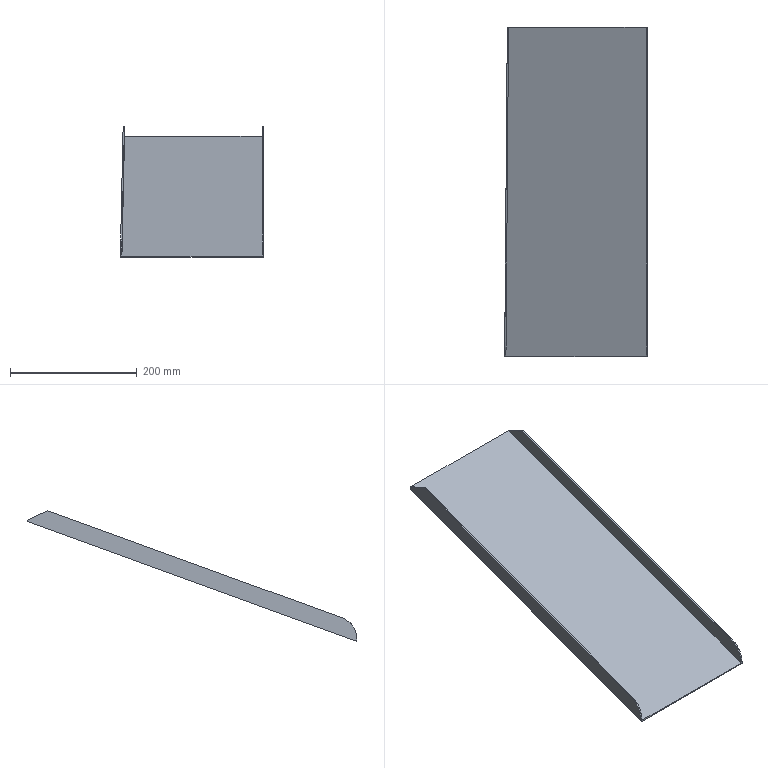Part | NX | features solid 2 | 1 solid | 14 faces | box 225.247 x 520 x 206.335 mm | volume 298449 mm3 | plane 8 | spline 5 | cylinder 1 | commonest cylinder face diameters 70 x1
STEP:
#1=CARTESIAN_POINT('',(-1188.242,-620.,-420.844));
#2=VERTEX_POINT('',#1);
#3=CARTESIAN_POINT('',(-967.,-620.,-420.844));
#4=VERTEX_POINT('',#3);
#5=CARTESIAN_POINT('',(-1490.,-620.,-420.844));
#6=DIRECTION('',(1.,0.,0.));
#7=VECTOR('',#6,1000.);
#8=LINE('',#5,#7);
#9=EDGE_CURVE('',#2,#4,#8,.T.);
#10=ORIENTED_EDGE('',*,*,#9,.T.);
#11=CARTESIAN_POINT('',(-967.,-100.,-231.58));
#12=VERTEX_POINT('',#11);
#13=CARTESIAN_POINT('',(-967.,-100.,-231.58));
#14=DIRECTION('',(0.,-0.9397,-0.342));
#15=VECTOR('',#14,1000.);
#16=LINE('',#13,#15);
#17=EDGE_CURVE('',#12,#4,#16,.T.);
#18=ORIENTED_EDGE('',*,*,#17,.F.);
#19=CARTESIAN_POINT('',(-1184.083,-100.019,-231.586));
#20=VERTEX_POINT('',#19);
#21=CARTESIAN_POINT('',(-1490.,-100.,-231.58));
#22=DIRECTION('',(1.,0.,0.));
#23=VECTOR('',#22,1000.);
#24=LINE('',#21,#23);
#25=EDGE_CURVE('',#20,#12,#24,.T.);
#26=ORIENTED_EDGE('',*,*,#25,.F.);
#27=CARTESIAN_POINT('',(-1188.242,-620.,-420.844));
#28=CARTESIAN_POINT('',(-1188.185,-612.224,-418.014));
#29=CARTESIAN_POINT('',(-1188.091,-599.128,-413.247));
#30=CARTESIAN_POINT('',(-1187.963,-581.34,-406.773));
#31=CARTESIAN_POINT('',(-1187.884,-570.46,-402.813));
#32=CARTESIAN_POINT('',(-1187.823,-561.941,-399.712));
#33=CARTESIAN_POINT('',(-1187.759,-553.064,-396.481));
#34=CARTESIAN_POINT('',(-1187.692,-543.828,-393.12));
#35=CARTESIAN_POINT('',(-1187.634,-535.833,-390.21));
#36=CARTESIAN_POINT('',(-1187.587,-529.258,-387.817));
#37=CARTESIAN_POINT('',(-1187.557,-525.074,-386.294));
#38=CARTESIAN_POINT('',(-1187.532,-521.683,-385.059));
#39=CARTESIAN_POINT('',(-1187.517,-519.544,-384.281));
#40=CARTESIAN_POINT('',(-1187.504,-517.822,-383.654));
#41=CARTESIAN_POINT('',(-1187.497,-516.74,-383.261));
#42=CARTESIAN_POINT('',(-1187.49,-515.874,-382.945));
#43=CARTESIAN_POINT('',(-1187.481,-514.573,-382.472));
#44=CARTESIAN_POINT('',(-1187.466,-512.553,-381.737));
#45=CARTESIAN_POINT('',(-1187.446,-509.692,-380.695));
#46=CARTESIAN_POINT('',(-1187.423,-506.519,-379.54));
#47=CARTESIAN_POINT('',(-1187.401,-503.548,-378.459));
#48=CARTESIAN_POINT('',(-1187.375,-499.877,-377.123));
#49=CARTESIAN_POINT('',(-1187.346,-495.82,-375.646));
#50=CARTESIAN_POINT('',(-1187.317,-491.809,-374.186));
#51=CARTESIAN_POINT('',(-1187.298,-489.18,-373.23));
#52=CARTESIAN_POINT('',(-1187.286,-487.505,-372.62));
#53=CARTESIAN_POINT('',(-1187.278,-486.462,-372.24));
#54=CARTESIAN_POINT('',(-1187.273,-485.772,-371.989));
#55=CARTESIAN_POINT('',(-1187.27,-485.382,-371.847));
#56=CARTESIAN_POINT('',(-1187.269,-485.186,-371.776));
#57=CARTESIAN_POINT('',(-1187.268,-485.054,-371.728));
#58=CARTESIAN_POINT('',(-1187.267,-484.948,-371.689));
#59=CARTESIAN_POINT('',(-1187.267,-484.886,-371.667));
#60=CARTESIAN_POINT('',(-1187.266,-484.815,-371.641));
#61=CARTESIAN_POINT('',(-1187.266,-484.839,-371.65));
#62=CARTESIAN_POINT('',(-1187.264,-484.524,-371.535));
#63=CARTESIAN_POINT('',(-1187.261,-484.132,-371.392));
#64=CARTESIAN_POINT('',(-1187.255,-483.245,-371.069));
#65=CARTESIAN_POINT('',(-1187.246,-482.064,-370.639));
#66=CARTESIAN_POINT('',(-1187.236,-480.662,-370.129));
#67=CARTESIAN_POINT('',(-1187.226,-479.309,-369.637));
#68=CARTESIAN_POINT('',(-1187.214,-477.558,-368.999));
#69=CARTESIAN_POINT('',(-1187.193,-474.64,-367.937));
#70=CARTESIAN_POINT('',(-1187.171,-471.638,-366.845));
#71=CARTESIAN_POINT('',(-1187.152,-468.97,-365.874));
#72=CARTESIAN_POINT('',(-1187.139,-467.136,-365.206));
#73=CARTESIAN_POINT('',(-1187.127,-465.468,-364.599));
#74=CARTESIAN_POINT('',(-1187.118,-464.216,-364.143));
#75=CARTESIAN_POINT('',(-1187.111,-463.299,-363.81));
#76=CARTESIAN_POINT('',(-1187.106,-462.652,-363.574));
#77=CARTESIAN_POINT('',(-1187.103,-462.15,-363.391));
#78=CARTESIAN_POINT('',(-1187.1,-461.811,-363.268));
#79=CARTESIAN_POINT('',(-1187.099,-461.632,-363.203));
#80=CARTESIAN_POINT('',(-1187.098,-461.5,-363.155));
#81=CARTESIAN_POINT('',(-1187.098,-461.448,-363.136));
#82=CARTESIAN_POINT('',(-1187.096,-461.203,-363.047));
#83=CARTESIAN_POINT('',(-1187.092,-460.733,-362.876));
#84=CARTESIAN_POINT('',(-1187.086,-459.849,-362.554));
#85=CARTESIAN_POINT('',(-1187.077,-458.631,-362.11));
#86=CARTESIAN_POINT('',(-1187.068,-457.276,-361.617));
#87=CARTESIAN_POINT('',(-1187.056,-455.599,-361.007));
#88=CARTESIAN_POINT('',(-1187.043,-453.755,-360.336));
#89=CARTESIAN_POINT('',(-1187.031,-451.936,-359.674));
#90=CARTESIAN_POINT('',(-1187.024,-450.764,-359.247));
#91=CARTESIAN_POINT('',(-1187.019,-450.,-358.969));
#92=CARTESIAN_POINT('',(-1187.017,-449.597,-358.822));
#93=CARTESIAN_POINT('',(-1187.015,-449.225,-358.687));
#94=CARTESIAN_POINT('',(-1187.012,-448.509,-358.427));
#95=CARTESIAN_POINT('',(-1187.006,-447.325,-357.995));
#96=CARTESIAN_POINT('',(-1186.998,-445.401,-357.295));
#97=CARTESIAN_POINT('',(-1186.989,-443.387,-356.562));
#98=CARTESIAN_POINT('',(-1186.982,-441.761,-355.97));
#99=CARTESIAN_POINT('',(-1186.977,-440.769,-355.609));
#100=CARTESIAN_POINT('',(-1186.974,-439.996,-355.328));
#101=CARTESIAN_POINT('',(-1186.971,-439.322,-355.083));
#102=CARTESIAN_POINT('',(-1186.969,-438.774,-354.883));
#103=CARTESIAN_POINT('',(-1186.967,-438.412,-354.751));
#104=CARTESIAN_POINT('',(-1186.966,-438.182,-354.668));
#105=CARTESIAN_POINT('',(-1186.965,-438.007,-354.604));
#106=CARTESIAN_POINT('',(-1186.965,-437.992,-354.598));
#107=CARTESIAN_POINT('',(-1186.965,-437.97,-354.59));
#108=CARTESIAN_POINT('',(-1186.965,-437.916,-354.571));
#109=CARTESIAN_POINT('',(-1186.964,-437.786,-354.524));
#110=CARTESIAN_POINT('',(-1186.963,-437.541,-354.434));
#111=CARTESIAN_POINT('',(-1186.96,-437.171,-354.3));
#112=CARTESIAN_POINT('',(-1186.957,-436.727,-354.138));
#113=CARTESIAN_POINT('',(-1186.952,-436.036,-353.886));
#114=CARTESIAN_POINT('',(-1186.945,-434.985,-353.504));
#115=CARTESIAN_POINT('',(-1186.933,-433.427,-352.937));
#116=CARTESIAN_POINT('',(-1186.918,-431.57,-352.261));
#117=CARTESIAN_POINT('',(-1186.901,-429.415,-351.477));
#118=CARTESIAN_POINT('',(-1186.881,-426.963,-350.584));
#119=CARTESIAN_POINT('',(-1186.858,-424.211,-349.583));
#120=CARTESIAN_POINT('',(-1186.837,-421.672,-348.659));
#121=CARTESIAN_POINT('',(-1186.819,-419.488,-347.864));
#122=CARTESIAN_POINT('',(-1186.807,-418.07,-347.348));
#123=CARTESIAN_POINT('',(-1186.797,-416.876,-346.913));
#124=CARTESIAN_POINT('',(-1186.792,-416.238,-346.681));
#125=CARTESIAN_POINT('',(-1186.788,-415.73,-346.496));
#126=CARTESIAN_POINT('',(-1186.786,-415.574,-346.439));
#127=CARTESIAN_POINT('',(-1186.784,-415.27,-346.328));
#128=CARTESIAN_POINT('',(-1186.779,-414.683,-346.115));
#129=CARTESIAN_POINT('',(-1186.772,-413.834,-345.806));
#130=CARTESIAN_POINT('',(-1186.761,-412.481,-345.313));
#131=CARTESIAN_POINT('',(-1186.747,-410.788,-344.697));
#132=CARTESIAN_POINT('',(-1186.713,-406.726,-343.218));
#133=CARTESIAN_POINT('',(-1186.68,-402.663,-341.74));
#134=CARTESIAN_POINT('',(-1186.647,-398.601,-340.261));
#135=CARTESIAN_POINT('',(-1186.626,-396.033,-339.327));
#136=CARTESIAN_POINT('',(-1186.589,-391.435,-337.653));
#137=CARTESIAN_POINT('',(-1186.537,-384.811,-335.242));
#138=CARTESIAN_POINT('',(-1186.484,-378.05,-332.781));
#139=CARTESIAN_POINT('',(-1186.441,-372.569,-330.787));
#140=CARTESIAN_POINT('',(-1186.415,-369.113,-329.528));
#141=CARTESIAN_POINT('',(-1186.394,-366.33,-328.516));
#142=CARTESIAN_POINT('',(-1186.378,-364.23,-327.751));
#143=CARTESIAN_POINT('',(-1186.364,-362.482,-327.115));
#144=CARTESIAN_POINT('',(-1186.355,-361.236,-326.662));
#145=CARTESIAN_POINT('',(-1186.35,-360.552,-326.413));
#146=CARTESIAN_POINT('',(-1186.345,-359.957,-326.196));
#147=CARTESIAN_POINT('',(-1186.343,-359.671,-326.092));
#148=CARTESIAN_POINT('',(-1186.339,-359.181,-325.914));
#149=CARTESIAN_POINT('',(-1186.333,-358.369,-325.618));
#150=CARTESIAN_POINT('',(-1186.324,-357.17,-325.182));
#151=CARTESIAN_POINT('',(-1186.313,-355.723,-324.655));
#152=CARTESIAN_POINT('',(-1186.298,-353.764,-323.942));
#153=CARTESIAN_POINT('',(-1186.279,-351.267,-323.033));
#154=CARTESIAN_POINT('',(-1186.247,-347.165,-321.54));
#155=CARTESIAN_POINT('',(-1186.206,-341.841,-319.603));
#156=CARTESIAN_POINT('',(-1186.153,-335.137,-317.162));
#157=CARTESIAN_POINT('',(-1186.097,-328.117,-314.607));
#158=CARTESIAN_POINT('',(-1186.018,-318.336,-311.047));
#159=CARTESIAN_POINT('',(-1185.912,-305.321,-306.31));
#160=CARTESIAN_POINT('',(-1185.773,-288.44,-300.166));
#161=CARTESIAN_POINT('',(-1185.647,-273.321,-294.663));
#162=CARTESIAN_POINT('',(-1185.54,-260.594,-290.031));
#163=CARTESIAN_POINT('',(-1185.47,-252.378,-287.041));
#164=CARTESIAN_POINT('',(-1185.413,-245.645,-284.59));
#165=CARTESIAN_POINT('',(-1185.369,-240.522,-282.725));
#166=CARTESIAN_POINT('',(-1185.332,-236.169,-281.141));
#167=CARTESIAN_POINT('',(-1185.302,-232.688,-279.874));
#168=CARTESIAN_POINT('',(-1185.279,-229.946,-278.876));
#169=CARTESIAN_POINT('',(-1185.259,-227.609,-278.025));
#170=CARTESIAN_POINT('',(-1185.232,-224.394,-276.855));
#171=CARTESIAN_POINT('',(-1185.185,-218.917,-274.862));
#172=CARTESIAN_POINT('',(-1185.12,-211.308,-272.092));
#173=CARTESIAN_POINT('',(-1185.045,-202.59,-268.919));
#174=CARTESIAN_POINT('',(-1184.973,-194.265,-265.889));
#175=CARTESIAN_POINT('',(-1184.905,-186.34,-263.005));
#176=CARTESIAN_POINT('',(-1184.851,-180.067,-260.721));
#177=CARTESIAN_POINT('',(-1184.809,-175.246,-258.967));
#178=CARTESIAN_POINT('',(-1184.779,-171.733,-257.688));
#179=CARTESIAN_POINT('',(-1184.754,-168.88,-256.65));
#180=CARTESIAN_POINT('',(-1184.737,-166.942,-255.944));
#181=CARTESIAN_POINT('',(-1184.728,-165.824,-255.537));
#182=CARTESIAN_POINT('',(-1184.721,-165.057,-255.258));
#183=CARTESIAN_POINT('',(-1184.712,-164.044,-254.89));
#184=CARTESIAN_POINT('',(-1184.701,-162.776,-254.428));
#185=CARTESIAN_POINT('',(-1184.681,-160.512,-253.604));
#186=CARTESIAN_POINT('',(-1184.641,-155.987,-251.957));
#187=CARTESIAN_POINT('',(-1184.581,-149.441,-249.575));
#188=CARTESIAN_POINT('',(-1184.506,-141.482,-246.678));
#189=CARTESIAN_POINT('',(-1184.402,-130.722,-242.761));
#190=CARTESIAN_POINT('',(-1184.264,-116.998,-237.766));
#191=CARTESIAN_POINT('',(-1184.145,-105.728,-233.664));
#192=CARTESIAN_POINT('',(-1184.083,-100.019,-231.586));
#193=B_SPLINE_CURVE_WITH_KNOTS('',3,(#27,#28,#29,#30,#31,#32,#33,#34,#35,#36,#37,#38,#39,#40,#41,#42,#43,#44,#45,#46,#47,#48,#49,#50,#51,#52,#53,#54,#55,#56,#57,#58,#59,#60,#61,#62,#63,#64,#65,#66,#67,#68,#69,#70,#71,#72,#73,#74,#75,#76,#77,#78,#79,#80,#81,#82,#83,#84,#85,#86,#87,#88,#89,#90,#91,#92,#93,#94,#95,#96,#97,#98,#99,#100,#101,#102,#103,#104,#105,#106,#107,#108,#109,#110,#111,#112,#113,#114,#115,#116,#117,#118,#119,#120,#121,#122,#123,#124,#125,#126,#127,#128,#129,#130,#131,#132,#133,#134,#135,#136,#137,#138,#139,#140,#141,#142,#143,#144,#145,#146,#147,#148,#149,#150,#151,#152,#153,#154,#155,#156,#157,#158,#159,#160,#161,#162,#163,#164,#165,#166,#167,#168,#169,#170,#171,#172,#173,#174,#175,#176,#177,#178,#179,#180,#181,#182,#183,#184,#185,#186,#187,#188,#189,#190,#191,#192),.UNSPECIFIED.,.F.,.F.,(4,1,1,1,1,1,1,1,1,1,1,1,1,1,1,1,1,1,1,1,1,1,1,1,1,1,1,1,1,1,1,1,1,1,1,1,1,1,1,1,1,1,1,1,1,1,1,1,1,1,1,1,1,1,1,1,1,1,1,1,1,1,1,1,1,1,1,1,1,1,1,1,1,1,1,1,1,1,1,1,1,1,1,1,1,1,1,1,1,1,1,1,1,1,1,1,1,1,1,1,1,1,1,1,1,1,1,1,1,1,1,1,1,1,1,1,1,1,1,1,1,1,1,1,1,1,1,1,1,1,1,1,1,1,1,1,1,1,1,1,1,1,1,1,1,1,1,1,1,1,1,1,1,1,1,1,1,1,1,1,1,1,1,4),(0.,0.0625,0.09375,0.1094,0.125,0.1406,0.1562,0.1719,0.1797,0.1875,0.1914,0.1953,0.1973,0.1992,0.2002,0.2012,0.2031,0.207,0.2109,0.2148,0.2188,0.2266,0.2344,0.2422,0.2461,0.25,0.2539,0.2559,0.2568,0.2578,0.2588,0.2593,0.2598,0.26,0.2603,0.2607,0.2617,0.2637,0.2656,0.2676,0.2695,0.2734,0.2812,0.2852,0.2891,0.293,0.2969,0.2988,0.3008,0.3027,0.3037,0.3042,0.3047,0.3049,0.3052,0.3057,0.3066,0.3086,0.3105,0.3125,0.3164,0.3203,0.3242,0.3262,0.3281,0.3301,0.332,0.3359,0.3398,0.3438,0.3457,0.3467,0.3477,0.3486,0.3491,0.3496,0.3499,0.35,0.3501,0.3503,0.3506,0.3516,0.3535,0.3555,0.3574,0.3594,0.3633,0.3672,0.3711,0.375,0.3789,0.3828,0.3867,0.3887,0.3906,0.3916,0.3926,0.3928,0.3931,0.3936,0.3945,0.3965,0.3984,0.4023,0.4062,0.4219,0.4258,0.4297,0.4375,0.4531,0.4688,0.4766,0.4844,0.4883,0.4922,0.4961,0.498,0.499,0.5,0.501,0.502,0.5039,0.5078,0.5117,0.5156,0.5234,0.5312,0.5469,0.5625,0.5781,0.5938,0.625,0.6562,0.6875,0.7031,0.7188,0.7266,0.7344,0.7422,0.7461,0.75,0.7539,0.7578,0.7656,0.7812,0.7969,0.8125,0.8281,0.8438,0.8516,0.8594,0.8672,0.8711,0.873,0.875,0.877,0.8789,0.8828,0.8906,0.9062,0.9219,0.9375,0.9688,1.),.UNSPECIFIED.);
#194=EDGE_CURVE('',#20,#2,#193,.F.);
#195=ORIENTED_EDGE('',*,*,#194,.T.);
#196=EDGE_LOOP('',(#10,#18,#26,#195));
#197=FACE_BOUND('',#196,.T.);
#198=CARTESIAN_POINT('',(-1490.,-63.022,-218.121));
#199=DIRECTION('',(0.,0.342,-0.9397));
#200=DIRECTION('',(-1.,0.,0.));
#201=AXIS2_PLACEMENT_3D('',#198,#199,#200);
#202=PLANE('',#201);
#203=ADVANCED_FACE('',(#197),#202,.F.);
#204=CARTESIAN_POINT('',(-965.,-620.,-418.747));
#205=VERTEX_POINT('',#204);
#206=CARTESIAN_POINT('',(-965.,-620.,-422.972));
#207=VERTEX_POINT('',#206);
#208=CARTESIAN_POINT('',(-965.,-620.,-570.));
#209=DIRECTION('',(0.,0.,-1.));
#210=VECTOR('',#209,1000.);
#211=LINE('',#208,#210);
#212=EDGE_CURVE('',#205,#207,#211,.T.);
#213=ORIENTED_EDGE('',*,*,#212,.F.);
#214=CARTESIAN_POINT('',(-967.,-620.,-418.747));
#215=VERTEX_POINT('',#214);
#216=CARTESIAN_POINT('',(50.,-620.,-418.747));
#217=DIRECTION('',(-1.,0.,0.));
#218=VECTOR('',#217,1000.);
#219=LINE('',#216,#218);
#220=EDGE_CURVE('',#205,#215,#219,.T.);
#221=ORIENTED_EDGE('',*,*,#220,.T.);
#222=CARTESIAN_POINT('',(-967.,-620.,-570.));
#223=DIRECTION('',(0.,0.,1.));
#224=VECTOR('',#223,1000.);
#225=LINE('',#222,#224);
#226=EDGE_CURVE('',#4,#215,#225,.T.);
#227=ORIENTED_EDGE('',*,*,#226,.F.);
#228=ORIENTED_EDGE('',*,*,#9,.F.);
#229=CARTESIAN_POINT('',(-1188.237,-620.,-418.747));
#230=VERTEX_POINT('',#229);
#231=CARTESIAN_POINT('',(-1188.242,-620.,-420.844));
#232=CARTESIAN_POINT('',(-1188.24,-620.,-420.145));
#233=CARTESIAN_POINT('',(-1188.238,-620.,-419.446));
#234=CARTESIAN_POINT('',(-1188.237,-620.,-418.747));
#235=B_SPLINE_CURVE_WITH_KNOTS('',3,(#231,#232,#233,#234),.UNSPECIFIED.,.F.,.F.,(4,4),(0.,0.002097),.UNSPECIFIED.);
#236=EDGE_CURVE('',#2,#230,#235,.T.);
#237=ORIENTED_EDGE('',*,*,#236,.T.);
#238=CARTESIAN_POINT('',(-1190.237,-620.,-418.747));
#239=VERTEX_POINT('',#238);
#240=CARTESIAN_POINT('',(-1188.237,-620.,-418.747));
#241=CARTESIAN_POINT('',(-1188.903,-620.,-418.747));
#242=CARTESIAN_POINT('',(-1189.57,-620.,-418.747));
#243=CARTESIAN_POINT('',(-1190.237,-620.,-418.747));
#244=B_SPLINE_CURVE_WITH_KNOTS('',3,(#240,#241,#242,#243),.UNSPECIFIED.,.F.,.F.,(4,4),(0.,0.002),.UNSPECIFIED.);
#245=EDGE_CURVE('',#230,#239,#244,.T.);
#246=ORIENTED_EDGE('',*,*,#245,.T.);
#247=CARTESIAN_POINT('',(-1190.247,-620.,-422.972));
#248=VERTEX_POINT('',#247);
#249=CARTESIAN_POINT('',(-1190.237,-620.,-418.747));
#250=CARTESIAN_POINT('',(-1190.24,-620.,-420.155));
#251=CARTESIAN_POINT('',(-1190.243,-620.,-421.564));
#252=CARTESIAN_POINT('',(-1190.247,-620.,-422.972));
#253=B_SPLINE_CURVE_WITH_KNOTS('',3,(#249,#250,#251,#252),.UNSPECIFIED.,.F.,.F.,(4,4),(-0.002097,0.002128),.UNSPECIFIED.);
#254=EDGE_CURVE('',#239,#248,#253,.T.);
#255=ORIENTED_EDGE('',*,*,#254,.T.);
#256=CARTESIAN_POINT('',(-1490.,-620.,-422.972));
#257=DIRECTION('',(1.,0.,0.));
#258=VECTOR('',#257,1000.);
#259=LINE('',#256,#258);
#260=EDGE_CURVE('',#248,#207,#259,.T.);
#261=ORIENTED_EDGE('',*,*,#260,.T.);
#262=EDGE_LOOP('',(#213,#221,#227,#228,#237,#246,#255,#261));
#263=FACE_BOUND('',#262,.T.);
#264=CARTESIAN_POINT('',(50.,-620.,-570.));
#265=DIRECTION('',(0.,1.,0.));
#266=DIRECTION('',(-1.,0.,0.));
#267=AXIS2_PLACEMENT_3D('',#264,#265,#266);
#268=PLANE('',#267);
#269=ADVANCED_FACE('',(#263),#268,.F.);
#270=CARTESIAN_POINT('',(-965.,-100.,-231.58));
#271=VERTEX_POINT('',#270);
#272=CARTESIAN_POINT('',(-965.,-100.,-233.708));
#273=VERTEX_POINT('',#272);
#274=CARTESIAN_POINT('',(-965.,-100.,0.));
#275=DIRECTION('',(0.,0.,-1.));
#276=VECTOR('',#275,1000.);
#277=LINE('',#274,#276);
#278=EDGE_CURVE('',#271,#273,#277,.T.);
#279=ORIENTED_EDGE('',*,*,#278,.F.);
#280=CARTESIAN_POINT('',(-965.,-132.043,-216.638));
#281=VERTEX_POINT('',#280);
#282=CARTESIAN_POINT('',(-965.,360.26,-446.202));
#283=DIRECTION('',(0.,0.9063,-0.4226));
#284=VECTOR('',#283,1000.);
#285=LINE('',#282,#284);
#286=EDGE_CURVE('',#271,#281,#285,.F.);
#287=ORIENTED_EDGE('',*,*,#286,.T.);
#288=CARTESIAN_POINT('',(-965.,-596.971,-385.858));
#289=VERTEX_POINT('',#288);
#290=CARTESIAN_POINT('',(-965.,-108.551,-208.087));
#291=DIRECTION('',(0.,-0.9397,-0.342));
#292=VECTOR('',#291,1000.);
#293=LINE('',#290,#292);
#294=EDGE_CURVE('',#281,#289,#293,.T.);
#295=ORIENTED_EDGE('',*,*,#294,.T.);
#296=CARTESIAN_POINT('',(-965.,-585.,-418.747));
#297=DIRECTION('',(1.,0.,0.));
#298=DIRECTION('',(0.,0.,-1.));
#299=AXIS2_PLACEMENT_3D('',#296,#297,#298);
#300=CIRCLE('',#299,35.);
#301=EDGE_CURVE('',#289,#205,#300,.T.);
#302=ORIENTED_EDGE('',*,*,#301,.T.);
#303=ORIENTED_EDGE('',*,*,#212,.T.);
#304=CARTESIAN_POINT('',(-965.,575.567,12.179));
#305=DIRECTION('',(0.,0.9397,0.342));
#306=VECTOR('',#305,1000.);
#307=LINE('',#304,#306);
#308=EDGE_CURVE('',#273,#207,#307,.F.);
#309=ORIENTED_EDGE('',*,*,#308,.F.);
#310=EDGE_LOOP('',(#279,#287,#295,#302,#303,#309));
#311=FACE_BOUND('',#310,.T.);
#312=CARTESIAN_POINT('',(-965.,574.883,14.058));
#313=DIRECTION('',(1.,0.,0.));
#314=DIRECTION('',(0.,0.,-1.));
#315=AXIS2_PLACEMENT_3D('',#312,#313,#314);
#316=PLANE('',#315);
#317=ADVANCED_FACE('',(#311),#316,.T.);
#318=CARTESIAN_POINT('',(-1186.09,-100.,-233.708));
#319=VERTEX_POINT('',#318);
#320=CARTESIAN_POINT('',(-1490.,-100.,-233.708));
#321=DIRECTION('',(1.,0.,0.));
#322=VECTOR('',#321,1000.);
#323=LINE('',#320,#322);
#324=EDGE_CURVE('',#319,#273,#323,.T.);
#325=ORIENTED_EDGE('',*,*,#324,.F.);
#326=CARTESIAN_POINT('',(-1186.083,-100.,-231.58));
#327=VERTEX_POINT('',#326);
#328=CARTESIAN_POINT('',(-1186.083,-100.,-231.58));
#329=CARTESIAN_POINT('',(-1186.085,-100.,-232.289));
#330=CARTESIAN_POINT('',(-1186.088,-100.,-232.998));
#331=CARTESIAN_POINT('',(-1186.09,-100.,-233.708));
#332=B_SPLINE_CURVE_WITH_KNOTS('',3,(#328,#329,#330,#331),.UNSPECIFIED.,.F.,.F.,(4,4),(0.,0.002128),.UNSPECIFIED.);
#333=EDGE_CURVE('',#327,#319,#332,.T.);
#334=ORIENTED_EDGE('',*,*,#333,.F.);
#335=CARTESIAN_POINT('',(-1186.083,-100.,-231.58));
#336=CARTESIAN_POINT('',(-1185.416,-100.,-231.58));
#337=CARTESIAN_POINT('',(-1184.749,-100.,-231.58));
#338=CARTESIAN_POINT('',(-1184.083,-100.,-231.58));
#339=B_SPLINE_CURVE_WITH_KNOTS('',3,(#335,#336,#337,#338),.UNSPECIFIED.,.F.,.F.,(4,4),(0.,1.),.UNSPECIFIED.);
#340=EDGE_CURVE('',#327,#20,#339,.T.);
#341=ORIENTED_EDGE('',*,*,#340,.T.);
#342=ORIENTED_EDGE('',*,*,#25,.T.);
#343=CARTESIAN_POINT('',(-965.,-100.,-231.58));
#344=DIRECTION('',(1.,0.,0.));
#345=VECTOR('',#344,1000.);
#346=LINE('',#343,#345);
#347=EDGE_CURVE('',#271,#12,#346,.F.);
#348=ORIENTED_EDGE('',*,*,#347,.F.);
#349=ORIENTED_EDGE('',*,*,#278,.T.);
#350=EDGE_LOOP('',(#325,#334,#341,#342,#348,#349));
#351=FACE_BOUND('',#350,.T.);
#352=CARTESIAN_POINT('',(2540.,-100.,0.));
#353=DIRECTION('',(0.,1.,0.));
#354=DIRECTION('',(0.,0.,1.));
#355=AXIS2_PLACEMENT_3D('',#352,#353,#354);
#356=PLANE('',#355);
#357=ADVANCED_FACE('',(#351),#356,.T.);
#358=CARTESIAN_POINT('',(-1186.09,-100.,-233.708));
#359=CARTESIAN_POINT('',(-1186.151,-105.657,-235.767));
#360=CARTESIAN_POINT('',(-1186.27,-116.851,-239.841));
#361=CARTESIAN_POINT('',(-1186.435,-133.279,-245.82));
#362=CARTESIAN_POINT('',(-1186.563,-146.678,-250.697));
#363=CARTESIAN_POINT('',(-1186.646,-155.88,-254.047));
#364=CARTESIAN_POINT('',(-1186.693,-161.123,-255.955));
#365=CARTESIAN_POINT('',(-1186.726,-164.949,-257.347));
#366=CARTESIAN_POINT('',(-1186.762,-169.075,-258.849));
#367=CARTESIAN_POINT('',(-1186.808,-174.471,-260.813));
#368=CARTESIAN_POINT('',(-1186.89,-183.963,-264.268));
#369=CARTESIAN_POINT('',(-1186.983,-194.79,-268.209));
#370=CARTESIAN_POINT('',(-1187.077,-205.624,-272.152));
#371=CARTESIAN_POINT('',(-1187.135,-212.395,-274.616));
#372=CARTESIAN_POINT('',(-1187.181,-217.811,-276.588));
#373=CARTESIAN_POINT('',(-1187.21,-221.197,-277.82));
#374=CARTESIAN_POINT('',(-1187.233,-223.906,-278.806));
#375=CARTESIAN_POINT('',(-1187.251,-225.935,-279.544));
#376=CARTESIAN_POINT('',(-1187.265,-227.634,-280.163));
#377=CARTESIAN_POINT('',(-1187.275,-228.807,-280.59));
#378=CARTESIAN_POINT('',(-1187.281,-229.503,-280.843));
#379=CARTESIAN_POINT('',(-1187.285,-229.953,-281.007));
#380=CARTESIAN_POINT('',(-1187.291,-230.676,-281.27));
#381=CARTESIAN_POINT('',(-1187.299,-231.543,-281.586));
#382=CARTESIAN_POINT('',(-1187.312,-233.1,-282.152));
#383=CARTESIAN_POINT('',(-1187.331,-235.289,-282.949));
#384=CARTESIAN_POINT('',(-1187.353,-237.906,-283.902));
#385=CARTESIAN_POINT('',(-1187.382,-241.366,-285.161));
#386=CARTESIAN_POINT('',(-1187.419,-245.642,-286.717));
#387=CARTESIAN_POINT('',(-1187.476,-252.377,-289.169));
#388=CARTESIAN_POINT('',(-1187.545,-260.598,-292.161));
#389=CARTESIAN_POINT('',(-1187.626,-270.148,-295.637));
#390=CARTESIAN_POINT('',(-1187.703,-279.38,-298.997));
#391=CARTESIAN_POINT('',(-1187.802,-291.269,-303.324));
#392=CARTESIAN_POINT('',(-1187.918,-305.338,-308.445));
#393=CARTESIAN_POINT('',(-1188.024,-318.352,-313.182));
#394=CARTESIAN_POINT('',(-1188.103,-328.13,-316.741));
#395=CARTESIAN_POINT('',(-1188.159,-335.148,-319.295));
#396=CARTESIAN_POINT('',(-1188.211,-341.848,-321.733));
#397=CARTESIAN_POINT('',(-1188.253,-347.168,-323.67));
#398=CARTESIAN_POINT('',(-1188.284,-351.266,-325.161));
#399=CARTESIAN_POINT('',(-1188.303,-353.761,-326.069));
#400=CARTESIAN_POINT('',(-1188.318,-355.719,-326.782));
#401=CARTESIAN_POINT('',(-1188.329,-357.164,-327.308));
#402=CARTESIAN_POINT('',(-1188.338,-358.361,-327.743));
#403=CARTESIAN_POINT('',(-1188.345,-359.173,-328.039));
#404=CARTESIAN_POINT('',(-1188.348,-359.661,-328.217));
#405=CARTESIAN_POINT('',(-1188.35,-359.953,-328.323));
#406=CARTESIAN_POINT('',(-1188.355,-360.518,-328.529));
#407=CARTESIAN_POINT('',(-1188.36,-361.177,-328.768));
#408=CARTESIAN_POINT('',(-1188.369,-362.373,-329.204));
#409=CARTESIAN_POINT('',(-1188.381,-364.06,-329.818));
#410=CARTESIAN_POINT('',(-1188.397,-366.093,-330.558));
#411=CARTESIAN_POINT('',(-1188.418,-368.801,-331.543));
#412=CARTESIAN_POINT('',(-1188.444,-372.186,-332.776));
#413=CARTESIAN_POINT('',(-1188.485,-377.603,-334.747));
#414=CARTESIAN_POINT('',(-1188.538,-384.374,-337.211));
#415=CARTESIAN_POINT('',(-1188.603,-392.499,-340.169));
#416=CARTESIAN_POINT('',(-1188.669,-400.624,-343.126));
#417=CARTESIAN_POINT('',(-1188.735,-408.749,-346.083));
#418=CARTESIAN_POINT('',(-1188.792,-415.52,-348.548));
#419=CARTESIAN_POINT('',(-1188.837,-420.936,-350.519));
#420=CARTESIAN_POINT('',(-1188.866,-424.322,-351.751));
#421=CARTESIAN_POINT('',(-1188.889,-427.03,-352.737));
#422=CARTESIAN_POINT('',(-1188.906,-429.061,-353.476));
#423=CARTESIAN_POINT('',(-1188.921,-430.754,-354.093));
#424=CARTESIAN_POINT('',(-1188.933,-432.107,-354.585));
#425=CARTESIAN_POINT('',(-1188.94,-432.957,-354.894));
#426=CARTESIAN_POINT('',(-1188.945,-433.544,-355.108));
#427=CARTESIAN_POINT('',(-1188.948,-433.891,-355.234));
#428=CARTESIAN_POINT('',(-1188.95,-434.081,-355.303));
#429=CARTESIAN_POINT('',(-1188.951,-434.294,-355.381));
#430=CARTESIAN_POINT('',(-1188.951,-434.288,-355.379));
#431=CARTESIAN_POINT('',(-1188.952,-434.328,-355.393));
#432=CARTESIAN_POINT('',(-1188.952,-434.427,-355.429));
#433=CARTESIAN_POINT('',(-1188.954,-434.715,-355.534));
#434=CARTESIAN_POINT('',(-1188.957,-435.446,-355.8));
#435=CARTESIAN_POINT('',(-1188.962,-436.601,-356.221));
#436=CARTESIAN_POINT('',(-1188.969,-438.175,-356.794));
#437=CARTESIAN_POINT('',(-1188.975,-439.568,-357.301));
#438=CARTESIAN_POINT('',(-1188.981,-440.896,-357.784));
#439=CARTESIAN_POINT('',(-1188.986,-442.082,-358.215));
#440=CARTESIAN_POINT('',(-1188.989,-442.825,-358.486));
#441=CARTESIAN_POINT('',(-1188.992,-443.541,-358.747));
#442=CARTESIAN_POINT('',(-1188.993,-443.929,-358.888));
#443=CARTESIAN_POINT('',(-1188.997,-444.65,-359.15));
#444=CARTESIAN_POINT('',(-1189.003,-446.013,-359.646));
#445=CARTESIAN_POINT('',(-1189.012,-447.859,-360.318));
#446=CARTESIAN_POINT('',(-1189.022,-449.875,-361.052));
#447=CARTESIAN_POINT('',(-1189.03,-451.244,-361.55));
#448=CARTESIAN_POINT('',(-1189.036,-452.099,-361.861));
#449=CARTESIAN_POINT('',(-1189.038,-452.44,-361.986));
#450=CARTESIAN_POINT('',(-1189.04,-452.719,-362.087));
#451=CARTESIAN_POINT('',(-1189.041,-452.893,-362.151));
#452=CARTESIAN_POINT('',(-1189.041,-452.867,-362.141));
#453=CARTESIAN_POINT('',(-1189.041,-452.934,-362.165));
#454=CARTESIAN_POINT('',(-1189.042,-453.039,-362.203));
#455=CARTESIAN_POINT('',(-1189.044,-453.311,-362.302));
#456=CARTESIAN_POINT('',(-1189.047,-453.681,-362.437));
#457=CARTESIAN_POINT('',(-1189.054,-454.639,-362.786));
#458=CARTESIAN_POINT('',(-1189.07,-456.868,-363.597));
#459=CARTESIAN_POINT('',(-1189.098,-460.757,-365.013));
#460=CARTESIAN_POINT('',(-1189.126,-464.72,-366.455));
#461=CARTESIAN_POINT('',(-1189.147,-467.539,-367.481));
#462=CARTESIAN_POINT('',(-1189.162,-469.719,-368.275));
#463=CARTESIAN_POINT('',(-1189.17,-470.827,-368.678));
#464=CARTESIAN_POINT('',(-1189.175,-471.519,-368.93));
#465=CARTESIAN_POINT('',(-1189.177,-471.771,-369.021));
#466=CARTESIAN_POINT('',(-1189.18,-472.236,-369.191));
#467=CARTESIAN_POINT('',(-1189.185,-472.897,-369.431));
#468=CARTESIAN_POINT('',(-1189.191,-473.751,-369.742));
#469=CARTESIAN_POINT('',(-1189.199,-474.764,-370.111));
#470=CARTESIAN_POINT('',(-1189.208,-476.12,-370.604));
#471=CARTESIAN_POINT('',(-1189.221,-477.812,-371.22));
#472=CARTESIAN_POINT('',(-1189.235,-479.843,-371.96));
#473=CARTESIAN_POINT('',(-1189.255,-482.552,-372.945));
#474=CARTESIAN_POINT('',(-1189.279,-485.937,-374.178));
#475=CARTESIAN_POINT('',(-1189.318,-491.354,-376.149));
#476=CARTESIAN_POINT('',(-1189.367,-498.125,-378.613));
#477=CARTESIAN_POINT('',(-1189.445,-508.958,-382.556));
#478=CARTESIAN_POINT('',(-1189.543,-522.5,-387.485));
#479=CARTESIAN_POINT('',(-1189.66,-538.75,-393.4));
#480=CARTESIAN_POINT('',(-1189.817,-560.417,-401.286));
#481=CARTESIAN_POINT('',(-1190.012,-587.5,-411.143));
#482=CARTESIAN_POINT('',(-1190.168,-609.167,-419.029));
#483=CARTESIAN_POINT('',(-1190.247,-620.,-422.972));
#484=B_SPLINE_CURVE_WITH_KNOTS('',3,(#358,#359,#360,#361,#362,#363,#364,#365,#366,#367,#368,#369,#370,#371,#372,#373,#374,#375,#376,#377,#378,#379,#380,#381,#382,#383,#384,#385,#386,#387,#388,#389,#390,#391,#392,#393,#394,#395,#396,#397,#398,#399,#400,#401,#402,#403,#404,#405,#406,#407,#408,#409,#410,#411,#412,#413,#414,#415,#416,#417,#418,#419,#420,#421,#422,#423,#424,#425,#426,#427,#428,#429,#430,#431,#432,#433,#434,#435,#436,#437,#438,#439,#440,#441,#442,#443,#444,#445,#446,#447,#448,#449,#450,#451,#452,#453,#454,#455,#456,#457,#458,#459,#460,#461,#462,#463,#464,#465,#466,#467,#468,#469,#470,#471,#472,#473,#474,#475,#476,#477,#478,#479,#480,#481,#482,#483),.UNSPECIFIED.,.F.,.F.,(4,1,1,1,1,1,1,1,1,1,1,1,1,1,1,1,1,1,1,1,1,1,1,1,1,1,1,1,1,1,1,1,1,1,1,1,1,1,1,1,1,1,1,1,1,1,1,1,1,1,1,1,1,1,1,1,1,1,1,1,1,1,1,1,1,1,1,1,1,1,1,1,1,1,1,1,1,1,1,1,1,1,1,1,1,1,1,1,1,1,1,1,1,1,1,1,1,1,1,1,1,1,1,1,1,1,1,1,1,1,1,1,1,1,1,1,1,1,1,1,1,1,1,4),(0.,0.03125,0.0625,0.09375,0.1094,0.1172,0.125,0.1328,0.1406,0.1562,0.1875,0.2031,0.2188,0.2266,0.2344,0.2383,0.2422,0.2461,0.248,0.249,0.25,0.251,0.252,0.2539,0.2578,0.2617,0.2656,0.2734,0.2812,0.2969,0.3125,0.3281,0.3438,0.375,0.4062,0.4219,0.4375,0.4531,0.4688,0.4766,0.4844,0.4883,0.4922,0.4961,0.498,0.499,0.5,0.501,0.502,0.5039,0.5078,0.5117,0.5156,0.5234,0.5312,0.5469,0.5625,0.5781,0.5938,0.6094,0.6172,0.625,0.6289,0.6328,0.6367,0.6387,0.6406,0.6416,0.6421,0.6426,0.6428,0.6431,0.6436,0.6445,0.6465,0.6484,0.6523,0.6543,0.6562,0.6582,0.6592,0.6602,0.6606,0.6611,0.6621,0.6641,0.668,0.6719,0.6758,0.6768,0.6777,0.6782,0.6787,0.6792,0.6797,0.6816,0.6836,0.6855,0.6875,0.6953,0.7031,0.707,0.7109,0.7129,0.7139,0.7144,0.7148,0.7158,0.7168,0.7188,0.7207,0.7227,0.7266,0.7305,0.7344,0.7422,0.75,0.7656,0.7812,0.8125,0.8438,0.875,0.9375,1.),.UNSPECIFIED.);
#485=EDGE_CURVE('',#319,#248,#484,.T.);
#486=ORIENTED_EDGE('',*,*,#485,.T.);
#487=ORIENTED_EDGE('',*,*,#254,.F.);
#488=CARTESIAN_POINT('',(-1190.014,-596.971,-385.858));
#489=VERTEX_POINT('',#488);
#490=CARTESIAN_POINT('',(-1190.237,-620.,-418.747));
#491=CARTESIAN_POINT('',(-1190.22,-620.,-411.562));
#492=CARTESIAN_POINT('',(-1190.174,-616.608,-400.951));
#493=CARTESIAN_POINT('',(-1190.086,-606.654,-390.561));
#494=CARTESIAN_POINT('',(-1190.038,-600.346,-387.086));
#495=CARTESIAN_POINT('',(-1190.014,-596.971,-385.858));
#496=B_SPLINE_CURVE_WITH_KNOTS('',3,(#490,#491,#492,#493,#494,#495),.UNSPECIFIED.,.F.,.F.,(4,1,1,4),(0.,0.02137,0.03205,0.04273),.UNSPECIFIED.);
#497=EDGE_CURVE('',#239,#489,#496,.T.);
#498=ORIENTED_EDGE('',*,*,#497,.T.);
#499=CARTESIAN_POINT('',(-1186.329,-132.042,-216.637));
#500=VERTEX_POINT('',#499);
#501=CARTESIAN_POINT('',(-1186.329,-132.042,-216.637));
#502=CARTESIAN_POINT('',(-1186.722,-170.785,-230.739));
#503=CARTESIAN_POINT('',(-1187.359,-248.273,-258.942));
#504=CARTESIAN_POINT('',(-1188.66,-403.25,-315.349));
#505=CARTESIAN_POINT('',(-1189.455,-519.482,-357.654));
#506=CARTESIAN_POINT('',(-1190.014,-596.971,-385.858));
#507=B_SPLINE_CURVE_WITH_KNOTS('',3,(#501,#502,#503,#504,#505,#506),.UNSPECIFIED.,.F.,.F.,(4,1,1,4),(0.,0.1237,0.2474,0.4948),.UNSPECIFIED.);
#508=EDGE_CURVE('',#500,#489,#507,.T.);
#509=ORIENTED_EDGE('',*,*,#508,.F.);
#510=CARTESIAN_POINT('',(-1186.329,-132.042,-216.637));
#511=CARTESIAN_POINT('',(-1186.25,-121.361,-221.618));
#512=CARTESIAN_POINT('',(-1186.167,-110.681,-226.599));
#513=CARTESIAN_POINT('',(-1186.083,-100.,-231.58));
#514=B_SPLINE_CURVE_WITH_KNOTS('',3,(#510,#511,#512,#513),.UNSPECIFIED.,.F.,.F.,(4,4),(0.09287,0.1282),.UNSPECIFIED.);
#515=EDGE_CURVE('',#500,#327,#514,.T.);
#516=ORIENTED_EDGE('',*,*,#515,.T.);
#517=ORIENTED_EDGE('',*,*,#333,.T.);
#518=EDGE_LOOP('',(#486,#487,#498,#509,#516,#517));
#519=FACE_BOUND('',#518,.T.);
#520=CARTESIAN_POINT('',(-1186.047,-105.288,-206.9));
#521=CARTESIAN_POINT('',(-1186.047,-96.053,-232.271));
#522=CARTESIAN_POINT('',(-1186.109,-110.986,-208.974));
#523=CARTESIAN_POINT('',(-1186.109,-101.752,-234.345));
#524=CARTESIAN_POINT('',(-1186.231,-122.344,-213.107));
#525=CARTESIAN_POINT('',(-1186.231,-113.109,-238.479));
#526=CARTESIAN_POINT('',(-1186.4,-138.962,-219.156));
#527=CARTESIAN_POINT('',(-1186.4,-129.728,-244.528));
#528=CARTESIAN_POINT('',(-1186.531,-152.519,-224.091));
#529=CARTESIAN_POINT('',(-1186.531,-143.285,-249.462));
#530=CARTESIAN_POINT('',(-1186.629,-163.177,-227.97));
#531=CARTESIAN_POINT('',(-1186.629,-153.942,-253.341));
#532=CARTESIAN_POINT('',(-1186.688,-169.768,-230.369));
#533=CARTESIAN_POINT('',(-1186.688,-160.533,-255.74));
#534=CARTESIAN_POINT('',(-1186.733,-174.981,-232.266));
#535=CARTESIAN_POINT('',(-1186.733,-165.747,-257.638));
#536=CARTESIAN_POINT('',(-1186.781,-180.497,-234.274));
#537=CARTESIAN_POINT('',(-1186.781,-171.262,-259.645));
#538=CARTESIAN_POINT('',(-1186.839,-187.288,-236.745));
#539=CARTESIAN_POINT('',(-1186.839,-178.053,-262.117));
#540=CARTESIAN_POINT('',(-1186.91,-195.481,-239.727));
#541=CARTESIAN_POINT('',(-1186.91,-186.247,-265.099));
#542=CARTESIAN_POINT('',(-1186.98,-203.663,-242.705));
#543=CARTESIAN_POINT('',(-1186.98,-194.428,-268.077));
#544=CARTESIAN_POINT('',(-1187.051,-211.847,-245.684));
#545=CARTESIAN_POINT('',(-1187.051,-202.613,-271.056));
#546=CARTESIAN_POINT('',(-1187.109,-218.667,-248.166));
#547=CARTESIAN_POINT('',(-1187.109,-209.433,-273.538));
#548=CARTESIAN_POINT('',(-1187.156,-224.123,-250.152));
#549=CARTESIAN_POINT('',(-1187.156,-214.889,-275.524));
#550=CARTESIAN_POINT('',(-1187.191,-228.215,-251.641));
#551=CARTESIAN_POINT('',(-1187.191,-218.98,-277.013));
#552=CARTESIAN_POINT('',(-1187.226,-232.308,-253.131));
#553=CARTESIAN_POINT('',(-1187.226,-223.074,-278.503));
#554=CARTESIAN_POINT('',(-1187.252,-235.373,-254.247));
#555=CARTESIAN_POINT('',(-1187.252,-226.138,-279.619));
#556=CARTESIAN_POINT('',(-1187.27,-237.425,-254.994));
#557=CARTESIAN_POINT('',(-1187.27,-228.19,-280.365));
#558=CARTESIAN_POINT('',(-1187.277,-238.267,-255.3));
#559=CARTESIAN_POINT('',(-1187.277,-229.032,-280.672));
#560=CARTESIAN_POINT('',(-1187.282,-238.883,-255.524));
#561=CARTESIAN_POINT('',(-1187.282,-229.648,-280.896));
#562=CARTESIAN_POINT('',(-1187.285,-239.193,-255.637));
#563=CARTESIAN_POINT('',(-1187.285,-229.958,-281.009));
#564=CARTESIAN_POINT('',(-1187.291,-239.892,-255.892));
#565=CARTESIAN_POINT('',(-1187.291,-230.658,-281.263));
#566=CARTESIAN_POINT('',(-1187.303,-241.313,-256.409));
#567=CARTESIAN_POINT('',(-1187.303,-232.079,-281.781));
#568=CARTESIAN_POINT('',(-1187.322,-243.548,-257.222));
#569=CARTESIAN_POINT('',(-1187.322,-234.314,-282.594));
#570=CARTESIAN_POINT('',(-1187.352,-247.063,-258.502));
#571=CARTESIAN_POINT('',(-1187.352,-237.829,-283.873));
#572=CARTESIAN_POINT('',(-1187.389,-251.418,-260.087));
#573=CARTESIAN_POINT('',(-1187.389,-242.184,-285.458));
#574=CARTESIAN_POINT('',(-1187.448,-258.273,-262.582));
#575=CARTESIAN_POINT('',(-1187.448,-249.038,-287.953));
#576=CARTESIAN_POINT('',(-1187.519,-266.642,-265.628));
#577=CARTESIAN_POINT('',(-1187.519,-257.408,-291.));
#578=CARTESIAN_POINT('',(-1187.628,-279.605,-270.346));
#579=CARTESIAN_POINT('',(-1187.628,-270.37,-295.717));
#580=CARTESIAN_POINT('',(-1187.757,-295.005,-275.951));
#581=CARTESIAN_POINT('',(-1187.757,-285.77,-301.323));
#582=CARTESIAN_POINT('',(-1187.899,-312.2,-282.21));
#583=CARTESIAN_POINT('',(-1187.899,-302.966,-307.581));
#584=CARTESIAN_POINT('',(-1188.007,-325.46,-287.036));
#585=CARTESIAN_POINT('',(-1188.007,-316.225,-312.407));
#586=CARTESIAN_POINT('',(-1188.087,-335.425,-290.663));
#587=CARTESIAN_POINT('',(-1188.087,-326.19,-316.034));
#588=CARTESIAN_POINT('',(-1188.144,-342.578,-293.266));
#589=CARTESIAN_POINT('',(-1188.144,-333.343,-318.638));
#590=CARTESIAN_POINT('',(-1188.198,-349.409,-295.753));
#591=CARTESIAN_POINT('',(-1188.198,-340.175,-321.124));
#592=CARTESIAN_POINT('',(-1188.241,-354.835,-297.727));
#593=CARTESIAN_POINT('',(-1188.241,-345.6,-323.099));
#594=CARTESIAN_POINT('',(-1188.273,-359.015,-299.249));
#595=CARTESIAN_POINT('',(-1188.273,-349.78,-324.62));
#596=CARTESIAN_POINT('',(-1188.296,-362.069,-300.361));
#597=CARTESIAN_POINT('',(-1188.296,-352.835,-325.732));
#598=CARTESIAN_POINT('',(-1188.315,-364.547,-301.262));
#599=CARTESIAN_POINT('',(-1188.315,-355.312,-326.634));
#600=CARTESIAN_POINT('',(-1188.33,-366.492,-301.97));
#601=CARTESIAN_POINT('',(-1188.33,-357.257,-327.342));
#602=CARTESIAN_POINT('',(-1188.339,-367.684,-302.404));
#603=CARTESIAN_POINT('',(-1188.339,-358.449,-327.776));
#604=CARTESIAN_POINT('',(-1188.346,-368.643,-302.753));
#605=CARTESIAN_POINT('',(-1188.346,-359.408,-328.125));
#606=CARTESIAN_POINT('',(-1188.351,-369.316,-302.998));
#607=CARTESIAN_POINT('',(-1188.351,-360.081,-328.37));
#608=CARTESIAN_POINT('',(-1188.36,-370.432,-303.404));
#609=CARTESIAN_POINT('',(-1188.36,-361.198,-328.776));
#610=CARTESIAN_POINT('',(-1188.37,-371.766,-303.89));
#611=CARTESIAN_POINT('',(-1188.37,-362.531,-329.261));
#612=CARTESIAN_POINT('',(-1188.383,-373.486,-304.516));
#613=CARTESIAN_POINT('',(-1188.383,-364.251,-329.887));
#614=CARTESIAN_POINT('',(-1188.404,-376.208,-305.506));
#615=CARTESIAN_POINT('',(-1188.404,-366.973,-330.878));
#616=CARTESIAN_POINT('',(-1188.43,-379.621,-306.749));
#617=CARTESIAN_POINT('',(-1188.43,-370.386,-332.12));
#618=CARTESIAN_POINT('',(-1188.472,-385.076,-308.734));
#619=CARTESIAN_POINT('',(-1188.472,-375.841,-334.106));
#620=CARTESIAN_POINT('',(-1188.525,-391.896,-311.217));
#621=CARTESIAN_POINT('',(-1188.525,-382.662,-336.588));
#622=CARTESIAN_POINT('',(-1188.59,-400.08,-314.195));
#623=CARTESIAN_POINT('',(-1188.59,-390.845,-339.567));
#624=CARTESIAN_POINT('',(-1188.656,-408.264,-317.174));
#625=CARTESIAN_POINT('',(-1188.656,-399.03,-342.546));
#626=CARTESIAN_POINT('',(-1188.723,-416.448,-320.153));
#627=CARTESIAN_POINT('',(-1188.723,-407.214,-345.524));
#628=CARTESIAN_POINT('',(-1188.779,-423.268,-322.635));
#629=CARTESIAN_POINT('',(-1188.779,-414.034,-348.007));
#630=CARTESIAN_POINT('',(-1188.825,-428.724,-324.621));
#631=CARTESIAN_POINT('',(-1188.825,-419.49,-349.993));
#632=CARTESIAN_POINT('',(-1188.854,-432.134,-325.862));
#633=CARTESIAN_POINT('',(-1188.854,-422.9,-351.234));
#634=CARTESIAN_POINT('',(-1188.877,-434.862,-326.855));
#635=CARTESIAN_POINT('',(-1188.877,-425.628,-352.227));
#636=CARTESIAN_POINT('',(-1188.895,-436.908,-327.6));
#637=CARTESIAN_POINT('',(-1188.895,-427.674,-352.971));
#638=CARTESIAN_POINT('',(-1188.909,-438.613,-328.22));
#639=CARTESIAN_POINT('',(-1188.909,-429.379,-353.592));
#640=CARTESIAN_POINT('',(-1188.921,-439.977,-328.717));
#641=CARTESIAN_POINT('',(-1188.921,-430.743,-354.088));
#642=CARTESIAN_POINT('',(-1188.93,-441.,-329.089));
#643=CARTESIAN_POINT('',(-1188.93,-431.765,-354.461));
#644=CARTESIAN_POINT('',(-1188.937,-441.853,-329.399));
#645=CARTESIAN_POINT('',(-1188.937,-432.619,-354.771));
#646=CARTESIAN_POINT('',(-1188.943,-442.534,-329.647));
#647=CARTESIAN_POINT('',(-1188.943,-433.299,-355.019));
#648=CARTESIAN_POINT('',(-1188.947,-442.964,-329.804));
#649=CARTESIAN_POINT('',(-1188.947,-433.729,-355.175));
#650=CARTESIAN_POINT('',(-1188.949,-443.297,-329.925));
#651=CARTESIAN_POINT('',(-1188.949,-434.063,-355.297));
#652=CARTESIAN_POINT('',(-1188.952,-443.576,-330.026));
#653=CARTESIAN_POINT('',(-1188.952,-434.341,-355.398));
#654=CARTESIAN_POINT('',(-1188.951,-443.527,-330.008));
#655=CARTESIAN_POINT('',(-1188.951,-434.292,-355.38));
#656=CARTESIAN_POINT('',(-1188.952,-443.598,-330.034));
#657=CARTESIAN_POINT('',(-1188.952,-434.363,-355.406));
#658=CARTESIAN_POINT('',(-1188.952,-443.679,-330.064));
#659=CARTESIAN_POINT('',(-1188.952,-434.445,-355.436));
#660=CARTESIAN_POINT('',(-1188.954,-444.015,-330.186));
#661=CARTESIAN_POINT('',(-1188.954,-434.781,-355.558));
#662=CARTESIAN_POINT('',(-1188.958,-444.904,-330.51));
#663=CARTESIAN_POINT('',(-1188.958,-435.67,-355.882));
#664=CARTESIAN_POINT('',(-1188.967,-446.956,-331.257));
#665=CARTESIAN_POINT('',(-1188.967,-437.721,-356.628));
#666=CARTESIAN_POINT('',(-1188.977,-449.359,-332.131));
#667=CARTESIAN_POINT('',(-1188.977,-440.125,-357.503));
#668=CARTESIAN_POINT('',(-1188.986,-451.295,-332.836));
#669=CARTESIAN_POINT('',(-1188.986,-442.061,-358.208));
#670=CARTESIAN_POINT('',(-1188.99,-452.227,-333.175));
#671=CARTESIAN_POINT('',(-1188.99,-442.993,-358.547));
#672=CARTESIAN_POINT('',(-1188.993,-452.936,-333.433));
#673=CARTESIAN_POINT('',(-1188.993,-443.701,-358.805));
#674=CARTESIAN_POINT('',(-1188.994,-453.35,-333.584));
#675=CARTESIAN_POINT('',(-1188.994,-444.115,-358.956));
#676=CARTESIAN_POINT('',(-1188.997,-453.986,-333.816));
#677=CARTESIAN_POINT('',(-1188.997,-444.752,-359.187));
#678=CARTESIAN_POINT('',(-1189.001,-454.766,-334.099));
#679=CARTESIAN_POINT('',(-1189.001,-445.531,-359.471));
#680=CARTESIAN_POINT('',(-1189.007,-456.112,-334.589));
#681=CARTESIAN_POINT('',(-1189.007,-446.877,-359.961));
#682=CARTESIAN_POINT('',(-1189.016,-457.899,-335.24));
#683=CARTESIAN_POINT('',(-1189.016,-448.665,-360.612));
#684=CARTESIAN_POINT('',(-1189.025,-459.535,-335.835));
#685=CARTESIAN_POINT('',(-1189.025,-450.3,-361.207));
#686=CARTESIAN_POINT('',(-1189.032,-460.733,-336.271));
#687=CARTESIAN_POINT('',(-1189.032,-451.499,-361.643));
#688=CARTESIAN_POINT('',(-1189.037,-461.469,-336.539));
#689=CARTESIAN_POINT('',(-1189.037,-452.234,-361.911));
#690=CARTESIAN_POINT('',(-1189.039,-461.877,-336.688));
#691=CARTESIAN_POINT('',(-1189.039,-452.643,-362.059));
#692=CARTESIAN_POINT('',(-1189.041,-462.114,-336.774));
#693=CARTESIAN_POINT('',(-1189.041,-452.88,-362.146));
#694=CARTESIAN_POINT('',(-1189.041,-462.087,-336.764));
#695=CARTESIAN_POINT('',(-1189.041,-452.852,-362.136));
#696=CARTESIAN_POINT('',(-1189.041,-462.132,-336.78));
#697=CARTESIAN_POINT('',(-1189.041,-452.897,-362.152));
#698=CARTESIAN_POINT('',(-1189.041,-462.167,-336.793));
#699=CARTESIAN_POINT('',(-1189.041,-452.932,-362.165));
#700=CARTESIAN_POINT('',(-1189.043,-462.343,-336.857));
#701=CARTESIAN_POINT('',(-1189.043,-453.108,-362.229));
#702=CARTESIAN_POINT('',(-1189.046,-462.793,-337.021));
#703=CARTESIAN_POINT('',(-1189.046,-453.558,-362.393));
#704=CARTESIAN_POINT('',(-1189.053,-463.832,-337.399));
#705=CARTESIAN_POINT('',(-1189.053,-454.597,-362.771));
#706=CARTESIAN_POINT('',(-1189.067,-465.787,-338.111));
#707=CARTESIAN_POINT('',(-1189.067,-456.553,-363.482));
#708=CARTESIAN_POINT('',(-1189.088,-468.605,-339.136));
#709=CARTESIAN_POINT('',(-1189.088,-459.37,-364.508));
#710=CARTESIAN_POINT('',(-1189.114,-472.278,-340.473));
#711=CARTESIAN_POINT('',(-1189.114,-463.044,-365.845));
#712=CARTESIAN_POINT('',(-1189.133,-474.941,-341.442));
#713=CARTESIAN_POINT('',(-1189.133,-465.706,-366.814));
#714=CARTESIAN_POINT('',(-1189.15,-477.267,-342.289));
#715=CARTESIAN_POINT('',(-1189.15,-468.033,-367.661));
#716=CARTESIAN_POINT('',(-1189.162,-478.852,-342.866));
#717=CARTESIAN_POINT('',(-1189.162,-469.618,-368.238));
#718=CARTESIAN_POINT('',(-1189.169,-479.926,-343.257));
#719=CARTESIAN_POINT('',(-1189.169,-470.691,-368.628));
#720=CARTESIAN_POINT('',(-1189.175,-480.683,-343.532));
#721=CARTESIAN_POINT('',(-1189.175,-471.448,-368.904));
#722=CARTESIAN_POINT('',(-1189.177,-480.96,-343.633));
#723=CARTESIAN_POINT('',(-1189.177,-471.725,-369.005));
#724=CARTESIAN_POINT('',(-1189.18,-481.417,-343.8));
#725=CARTESIAN_POINT('',(-1189.18,-472.183,-369.171));
#726=CARTESIAN_POINT('',(-1189.185,-482.087,-344.043));
#727=CARTESIAN_POINT('',(-1189.185,-472.852,-369.415));
#728=CARTESIAN_POINT('',(-1189.191,-482.946,-344.356));
#729=CARTESIAN_POINT('',(-1189.191,-473.711,-369.728));
#730=CARTESIAN_POINT('',(-1189.201,-484.307,-344.851));
#731=CARTESIAN_POINT('',(-1189.201,-475.073,-370.223));
#732=CARTESIAN_POINT('',(-1189.213,-486.013,-345.472));
#733=CARTESIAN_POINT('',(-1189.213,-476.779,-370.844));
#734=CARTESIAN_POINT('',(-1189.228,-488.059,-346.217));
#735=CARTESIAN_POINT('',(-1189.228,-478.825,-371.589));
#736=CARTESIAN_POINT('',(-1189.248,-490.787,-347.21));
#737=CARTESIAN_POINT('',(-1189.248,-481.553,-372.582));
#738=CARTESIAN_POINT('',(-1189.272,-494.197,-348.451));
#739=CARTESIAN_POINT('',(-1189.272,-484.963,-373.823));
#740=CARTESIAN_POINT('',(-1189.302,-498.29,-349.941));
#741=CARTESIAN_POINT('',(-1189.302,-489.055,-375.312));
#742=CARTESIAN_POINT('',(-1189.331,-502.382,-351.43));
#743=CARTESIAN_POINT('',(-1189.331,-493.147,-376.802));
#744=CARTESIAN_POINT('',(-1189.371,-507.838,-353.416));
#745=CARTESIAN_POINT('',(-1189.371,-498.603,-378.788));
#746=CARTESIAN_POINT('',(-1189.44,-517.385,-356.891));
#747=CARTESIAN_POINT('',(-1189.44,-508.151,-382.263));
#748=CARTESIAN_POINT('',(-1189.538,-531.026,-361.856));
#749=CARTESIAN_POINT('',(-1189.538,-521.791,-387.227));
#750=CARTESIAN_POINT('',(-1189.656,-547.394,-367.813));
#751=CARTESIAN_POINT('',(-1189.656,-538.16,-393.185));
#752=CARTESIAN_POINT('',(-1189.814,-569.218,-375.757));
#753=CARTESIAN_POINT('',(-1189.814,-559.984,-401.128));
#754=CARTESIAN_POINT('',(-1190.01,-596.499,-385.686));
#755=CARTESIAN_POINT('',(-1190.01,-587.264,-411.058));
#756=CARTESIAN_POINT('',(-1190.168,-618.323,-393.629));
#757=CARTESIAN_POINT('',(-1190.168,-609.088,-419.001));
#758=CARTESIAN_POINT('',(-1190.247,-629.235,-397.601));
#759=CARTESIAN_POINT('',(-1190.247,-620.,-422.972));
#760=B_SPLINE_SURFACE_WITH_KNOTS('',3,1,((#520,#521),(#522,#523),(#524,#525),(#526,#527),(#528,#529),(#530,#531),(#532,#533),(#534,#535),(#536,#537),(#538,#539),(#540,#541),(#542,#543),(#544,#545),(#546,#547),(#548,#549),(#550,#551),(#552,#553),(#554,#555),(#556,#557),(#558,#559),(#560,#561),(#562,#563),(#564,#565),(#566,#567),(#568,#569),(#570,#571),(#572,#573),(#574,#575),(#576,#577),(#578,#579),(#580,#581),(#582,#583),(#584,#585),(#586,#587),(#588,#589),(#590,#591),(#592,#593),(#594,#595),(#596,#597),(#598,#599),(#600,#601),(#602,#603),(#604,#605),(#606,#607),(#608,#609),(#610,#611),(#612,#613),(#614,#615),(#616,#617),(#618,#619),(#620,#621),(#622,#623),(#624,#625),(#626,#627),(#628,#629),(#630,#631),(#632,#633),(#634,#635),(#636,#637),(#638,#639),(#640,#641),(#642,#643),(#644,#645),(#646,#647),(#648,#649),(#650,#651),(#652,#653),(#654,#655),(#656,#657),(#658,#659),(#660,#661),(#662,#663),(#664,#665),(#666,#667),(#668,#669),(#670,#671),(#672,#673),(#674,#675),(#676,#677),(#678,#679),(#680,#681),(#682,#683),(#684,#685),(#686,#687),(#688,#689),(#690,#691),(#692,#693),(#694,#695),(#696,#697),(#698,#699),(#700,#701),(#702,#703),(#704,#705),(#706,#707),(#708,#709),(#710,#711),(#712,#713),(#714,#715),(#716,#717),(#718,#719),(#720,#721),(#722,#723),(#724,#725),(#726,#727),(#728,#729),(#730,#731),(#732,#733),(#734,#735),(#736,#737),(#738,#739),(#740,#741),(#742,#743),(#744,#745),(#746,#747),(#748,#749),(#750,#751),(#752,#753),(#754,#755),(#756,#757),(#758,#759)),.SURF_OF_LINEAR_EXTRUSION.,.F.,.F.,.F.,(4,1,1,1,1,1,1,1,1,1,1,1,1,1,1,1,1,1,1,1,1,1,1,1,1,1,1,1,1,1,1,1,1,1,1,1,1,1,1,1,1,1,1,1,1,1,1,1,1,1,1,1,1,1,1,1,1,1,1,1,1,1,1,1,1,1,1,1,1,1,1,1,1,1,1,1,1,1,1,1,1,1,1,1,1,1,1,1,1,1,1,1,1,1,1,1,1,1,1,1,1,1,1,1,1,1,1,1,1,1,1,1,1,1,1,1,1,4),(2,2),(-0.007267,0.02421,0.05569,0.08716,0.1029,0.1186,0.1265,0.1344,0.1501,0.1659,0.1816,0.1973,0.2131,0.2209,0.2288,0.2367,0.2445,0.2465,0.2485,0.2495,0.25,0.2505,0.2524,0.2564,0.2603,0.2682,0.276,0.2918,0.3075,0.339,0.3705,0.4019,0.4177,0.4334,0.4492,0.4649,0.4728,0.4806,0.4885,0.4924,0.4964,0.4983,0.5003,0.5023,0.5042,0.5082,0.5121,0.52,0.5278,0.5436,0.5593,0.5751,0.5908,0.6065,0.6144,0.6223,0.6262,0.6301,0.6341,0.636,0.638,0.64,0.641,0.6419,0.6424,0.6429,0.6434,0.6439,0.6449,0.6459,0.6498,0.6538,0.6577,0.6597,0.6601,0.6606,0.6616,0.6626,0.6636,0.6656,0.6695,0.6734,0.6754,0.6774,0.6783,0.6786,0.6788,0.6793,0.6803,0.6813,0.6852,0.6892,0.6931,0.701,0.7049,0.7088,0.7108,0.7128,0.7138,0.7142,0.7147,0.7157,0.7167,0.7187,0.7206,0.7246,0.7285,0.7324,0.7403,0.7482,0.7561,0.7639,0.7797,0.8111,0.8426,0.8741,0.937,1.),(0.,1.),.UNSPECIFIED.);
#761=ADVANCED_FACE('',(#519),#760,.F.);
#762=ORIENTED_EDGE('',*,*,#260,.F.);
#763=ORIENTED_EDGE('',*,*,#485,.F.);
#764=ORIENTED_EDGE('',*,*,#324,.T.);
#765=ORIENTED_EDGE('',*,*,#308,.T.);
#766=EDGE_LOOP('',(#762,#763,#764,#765));
#767=FACE_BOUND('',#766,.T.);
#768=CARTESIAN_POINT('',(-1490.,-62.338,-220.));
#769=DIRECTION('',(0.,0.342,-0.9397));
#770=DIRECTION('',(-1.,0.,0.));
#771=AXIS2_PLACEMENT_3D('',#768,#769,#770);
#772=PLANE('',#771);
#773=ADVANCED_FACE('',(#767),#772,.T.);
#774=CARTESIAN_POINT('',(-1184.328,-132.061,-216.644));
#775=VERTEX_POINT('',#774);
#776=CARTESIAN_POINT('',(-1188.014,-596.971,-385.858));
#777=VERTEX_POINT('',#776);
#778=CARTESIAN_POINT('',(-1184.327,-132.061,-216.644));
#779=CARTESIAN_POINT('',(-1184.714,-170.801,-230.744));
#780=CARTESIAN_POINT('',(-1185.363,-248.287,-258.947));
#781=CARTESIAN_POINT('',(-1186.658,-403.254,-315.351));
#782=CARTESIAN_POINT('',(-1187.455,-519.485,-357.655));
#783=CARTESIAN_POINT('',(-1188.014,-596.971,-385.858));
#784=B_SPLINE_CURVE_WITH_KNOTS('',3,(#778,#779,#780,#781,#782,#783),.UNSPECIFIED.,.F.,.F.,(4,1,1,4),(0.04518,0.2687,0.4922,0.9392),.UNSPECIFIED.);
#785=EDGE_CURVE('',#775,#777,#784,.T.);
#786=ORIENTED_EDGE('',*,*,#785,.F.);
#787=CARTESIAN_POINT('',(-1184.328,-132.061,-216.644));
#788=CARTESIAN_POINT('',(-1184.995,-132.054,-216.642));
#789=CARTESIAN_POINT('',(-1185.662,-132.048,-216.64));
#790=CARTESIAN_POINT('',(-1186.329,-132.042,-216.637));
#791=B_SPLINE_CURVE_WITH_KNOTS('',3,(#787,#788,#789,#790),.UNSPECIFIED.,.F.,.F.,(4,4),(0.0005989,1.001),.UNSPECIFIED.);
#792=EDGE_CURVE('',#775,#500,#791,.T.);
#793=ORIENTED_EDGE('',*,*,#792,.T.);
#794=ORIENTED_EDGE('',*,*,#508,.T.);
#795=CARTESIAN_POINT('',(-1190.014,-596.971,-385.858));
#796=CARTESIAN_POINT('',(-1189.347,-596.971,-385.858));
#797=CARTESIAN_POINT('',(-1188.68,-596.971,-385.858));
#798=CARTESIAN_POINT('',(-1188.014,-596.971,-385.858));
#799=B_SPLINE_CURVE_WITH_KNOTS('',3,(#795,#796,#797,#798),.UNSPECIFIED.,.F.,.F.,(4,4),(0.,0.002),.UNSPECIFIED.);
#800=EDGE_CURVE('',#489,#777,#799,.T.);
#801=ORIENTED_EDGE('',*,*,#800,.T.);
#802=EDGE_LOOP('',(#786,#793,#794,#801));
#803=FACE_BOUND('',#802,.T.);
#804=CARTESIAN_POINT('',(-1184.299,-129.27,-215.628));
#805=CARTESIAN_POINT('',(-1184.666,-165.7,-228.888));
#806=CARTESIAN_POINT('',(-1184.968,-202.132,-242.148));
#807=CARTESIAN_POINT('',(-1185.65,-281.897,-271.18));
#808=CARTESIAN_POINT('',(-1186.019,-325.229,-286.952));
#809=CARTESIAN_POINT('',(-1186.509,-390.229,-310.61));
#810=CARTESIAN_POINT('',(-1186.682,-411.897,-318.496));
#811=CARTESIAN_POINT('',(-1186.912,-438.981,-328.354));
#812=CARTESIAN_POINT('',(-1186.956,-444.39,-330.323));
#813=CARTESIAN_POINT('',(-1187.002,-455.224,-334.266));
#814=CARTESIAN_POINT('',(-1187.03,-460.646,-336.239));
#815=CARTESIAN_POINT('',(-1187.147,-476.896,-342.154));
#816=CARTESIAN_POINT('',(-1187.226,-487.729,-346.097));
#817=CARTESIAN_POINT('',(-1187.547,-532.299,-362.319));
#818=CARTESIAN_POINT('',(-1187.791,-566.036,-374.598));
#819=CARTESIAN_POINT('',(-1188.034,-599.773,-386.878));
#820=CARTESIAN_POINT('',(-1186.299,-129.252,-215.622));
#821=CARTESIAN_POINT('',(-1186.666,-165.684,-228.882));
#822=CARTESIAN_POINT('',(-1186.968,-202.117,-242.143));
#823=CARTESIAN_POINT('',(-1187.65,-281.882,-271.175));
#824=CARTESIAN_POINT('',(-1188.019,-325.216,-286.947));
#825=CARTESIAN_POINT('',(-1188.509,-390.216,-310.605));
#826=CARTESIAN_POINT('',(-1188.682,-411.883,-318.491));
#827=CARTESIAN_POINT('',(-1188.912,-438.966,-328.349));
#828=CARTESIAN_POINT('',(-1188.956,-444.382,-330.32));
#829=CARTESIAN_POINT('',(-1189.002,-455.216,-334.263));
#830=CARTESIAN_POINT('',(-1189.03,-460.633,-336.235));
#831=CARTESIAN_POINT('',(-1189.147,-476.883,-342.149));
#832=CARTESIAN_POINT('',(-1189.225,-487.716,-346.092));
#833=CARTESIAN_POINT('',(-1189.547,-532.287,-362.315));
#834=CARTESIAN_POINT('',(-1189.79,-566.023,-374.594));
#835=CARTESIAN_POINT('',(-1190.034,-599.76,-386.873));
#836=CARTESIAN_POINT('',(-1186.317,-129.252,-215.622));
#837=CARTESIAN_POINT('',(-1186.684,-165.684,-228.882));
#838=CARTESIAN_POINT('',(-1186.986,-202.117,-242.143));
#839=CARTESIAN_POINT('',(-1187.668,-281.882,-271.175));
#840=CARTESIAN_POINT('',(-1188.037,-325.216,-286.947));
#841=CARTESIAN_POINT('',(-1188.527,-390.216,-310.605));
#842=CARTESIAN_POINT('',(-1188.7,-411.882,-318.491));
#843=CARTESIAN_POINT('',(-1188.93,-438.966,-328.348));
#844=CARTESIAN_POINT('',(-1188.974,-444.382,-330.32));
#845=CARTESIAN_POINT('',(-1189.021,-455.216,-334.263));
#846=CARTESIAN_POINT('',(-1189.049,-460.633,-336.235));
#847=CARTESIAN_POINT('',(-1189.166,-476.883,-342.149));
#848=CARTESIAN_POINT('',(-1189.244,-487.716,-346.092));
#849=CARTESIAN_POINT('',(-1189.565,-532.286,-362.314));
#850=CARTESIAN_POINT('',(-1189.809,-566.023,-374.594));
#851=CARTESIAN_POINT('',(-1190.052,-599.76,-386.873));
#852=B_SPLINE_SURFACE_WITH_KNOTS('',1,3,((#804,#805,#806,#807,#808,#809,#810,#811,#812,#813,#814,#815,#816,#817,#818,#819),(#820,#821,#822,#823,#824,#825,#826,#827,#828,#829,#830,#831,#832,#833,#834,#835),(#836,#837,#838,#839,#840,#841,#842,#843,#844,#845,#846,#847,#848,#849,#850,#851)),.RULED_SURF.,.F.,.F.,.F.,(2,1,2),(4,2,2,2,2,2,2,4),(0.,1.,1.009),(0.03981,0.25,0.5,0.625,0.6562,0.6875,0.75,0.9446),.UNSPECIFIED.);
#853=ADVANCED_FACE('',(#803),#852,.T.);
#854=ORIENTED_EDGE('',*,*,#194,.F.);
#855=CARTESIAN_POINT('',(-1184.333,-132.061,-216.644));
#856=CARTESIAN_POINT('',(-1184.248,-121.38,-221.625));
#857=CARTESIAN_POINT('',(-1184.164,-110.7,-226.606));
#858=CARTESIAN_POINT('',(-1184.079,-100.019,-231.586));
#859=B_SPLINE_CURVE_WITH_KNOTS('',3,(#855,#856,#857,#858),.UNSPECIFIED.,.F.,.F.,(4,4),(0.,1.),.UNSPECIFIED.);
#860=EDGE_CURVE('',#20,#775,#859,.F.);
#861=ORIENTED_EDGE('',*,*,#860,.T.);
#862=ORIENTED_EDGE('',*,*,#785,.T.);
#863=CARTESIAN_POINT('',(-1188.014,-596.971,-385.858));
#864=CARTESIAN_POINT('',(-1188.038,-600.348,-387.087));
#865=CARTESIAN_POINT('',(-1188.086,-606.607,-390.527));
#866=CARTESIAN_POINT('',(-1188.152,-614.104,-398.334));
#867=CARTESIAN_POINT('',(-1188.205,-618.886,-408.008));
#868=CARTESIAN_POINT('',(-1188.228,-620.,-415.153));
#869=CARTESIAN_POINT('',(-1188.237,-620.,-418.747));
#870=B_SPLINE_CURVE_WITH_KNOTS('',3,(#863,#864,#865,#866,#867,#868,#869),.UNSPECIFIED.,.F.,.F.,(4,1,1,1,4),(0.,0.01063,0.02126,0.03189,0.04252),.UNSPECIFIED.);
#871=EDGE_CURVE('',#777,#230,#870,.T.);
#872=ORIENTED_EDGE('',*,*,#871,.T.);
#873=ORIENTED_EDGE('',*,*,#236,.F.);
#874=EDGE_LOOP('',(#854,#861,#862,#872,#873));
#875=FACE_BOUND('',#874,.T.);
#876=CARTESIAN_POINT('',(-1184.083,-100.019,-231.586));
#877=CARTESIAN_POINT('',(-1184.083,-108.57,-208.094));
#878=CARTESIAN_POINT('',(-1184.552,-143.35,-247.358));
#879=CARTESIAN_POINT('',(-1184.552,-151.9,-223.865));
#880=CARTESIAN_POINT('',(-1185.29,-230.014,-278.901));
#881=CARTESIAN_POINT('',(-1185.29,-238.565,-255.408));
#882=CARTESIAN_POINT('',(-1186.161,-338.343,-318.329));
#883=CARTESIAN_POINT('',(-1186.161,-346.894,-294.837));
#884=CARTESIAN_POINT('',(-1186.89,-425.015,-349.875));
#885=CARTESIAN_POINT('',(-1186.89,-433.565,-326.383));
#886=CARTESIAN_POINT('',(-1187.427,-511.677,-381.418));
#887=CARTESIAN_POINT('',(-1187.427,-520.227,-357.925));
#888=CARTESIAN_POINT('',(-1187.929,-576.679,-405.077));
#889=CARTESIAN_POINT('',(-1187.929,-585.23,-381.584));
#890=CARTESIAN_POINT('',(-1188.242,-620.013,-420.849));
#891=CARTESIAN_POINT('',(-1188.242,-628.563,-397.356));
#892=B_SPLINE_SURFACE_WITH_KNOTS('',3,1,((#876,#877),(#878,#879),(#880,#881),(#882,#883),(#884,#885),(#886,#887),(#888,#889),(#890,#891)),.SURF_OF_LINEAR_EXTRUSION.,.F.,.F.,.F.,(4,1,1,1,1,4),(2,2),(0.,0.25,0.5,0.625,0.75,1.),(0.,1.),.UNSPECIFIED.);
#893=ADVANCED_FACE('',(#875),#892,.F.);
#894=ORIENTED_EDGE('',*,*,#294,.F.);
#895=CARTESIAN_POINT('',(-967.,-132.043,-216.638));
#896=VERTEX_POINT('',#895);
#897=CARTESIAN_POINT('',(-965.,-132.043,-216.638));
#898=DIRECTION('',(-1.,0.,0.));
#899=VECTOR('',#898,1000.);
#900=LINE('',#897,#899);
#901=EDGE_CURVE('',#281,#896,#900,.T.);
#902=ORIENTED_EDGE('',*,*,#901,.T.);
#903=CARTESIAN_POINT('',(-967.,-596.971,-385.858));
#904=VERTEX_POINT('',#903);
#905=CARTESIAN_POINT('',(-967.,-108.551,-208.087));
#906=DIRECTION('',(0.,-0.9397,-0.342));
#907=VECTOR('',#906,1000.);
#908=LINE('',#905,#907);
#909=EDGE_CURVE('',#896,#904,#908,.T.);
#910=ORIENTED_EDGE('',*,*,#909,.T.);
#911=CARTESIAN_POINT('',(-965.,-596.971,-385.858));
#912=DIRECTION('',(-1.,0.,0.));
#913=VECTOR('',#912,1000.);
#914=LINE('',#911,#913);
#915=EDGE_CURVE('',#904,#289,#914,.F.);
#916=ORIENTED_EDGE('',*,*,#915,.T.);
#917=EDGE_LOOP('',(#894,#902,#910,#916));
#918=FACE_BOUND('',#917,.T.);
#919=CARTESIAN_POINT('',(-965.,-108.551,-208.087));
#920=DIRECTION('',(0.,0.342,-0.9397));
#921=DIRECTION('',(0.,-0.9397,-0.342));
#922=AXIS2_PLACEMENT_3D('',#919,#920,#921);
#923=PLANE('',#922);
#924=ADVANCED_FACE('',(#918),#923,.F.);
#925=ORIENTED_EDGE('',*,*,#909,.F.);
#926=CARTESIAN_POINT('',(-967.,-100.,-231.58));
#927=DIRECTION('',(0.,-0.9063,0.4226));
#928=VECTOR('',#927,1000.);
#929=LINE('',#926,#928);
#930=EDGE_CURVE('',#896,#12,#929,.F.);
#931=ORIENTED_EDGE('',*,*,#930,.T.);
#932=ORIENTED_EDGE('',*,*,#17,.T.);
#933=ORIENTED_EDGE('',*,*,#226,.T.);
#934=CARTESIAN_POINT('',(-967.,-585.,-418.747));
#935=DIRECTION('',(-1.,0.,0.));
#936=DIRECTION('',(0.,0.,1.));
#937=AXIS2_PLACEMENT_3D('',#934,#935,#936);
#938=CIRCLE('',#937,35.);
#939=EDGE_CURVE('',#215,#904,#938,.T.);
#940=ORIENTED_EDGE('',*,*,#939,.T.);
#941=EDGE_LOOP('',(#925,#931,#932,#933,#940));
#942=FACE_BOUND('',#941,.T.);
#943=CARTESIAN_POINT('',(-967.,-100.,-231.58));
#944=DIRECTION('',(-1.,0.,0.));
#945=DIRECTION('',(0.,0.,1.));
#946=AXIS2_PLACEMENT_3D('',#943,#944,#945);
#947=PLANE('',#946);
#948=ADVANCED_FACE('',(#942),#947,.T.);
#949=ORIENTED_EDGE('',*,*,#497,.F.);
#950=ORIENTED_EDGE('',*,*,#245,.F.);
#951=ORIENTED_EDGE('',*,*,#871,.F.);
#952=ORIENTED_EDGE('',*,*,#800,.F.);
#953=EDGE_LOOP('',(#949,#950,#951,#952));
#954=FACE_BOUND('',#953,.T.);
#955=CARTESIAN_POINT('',(-1190.25,-620.,-418.747));
#956=CARTESIAN_POINT('',(-1190.25,-620.,-394.24));
#957=CARTESIAN_POINT('',(-1190.25,-596.971,-385.858));
#958=CARTESIAN_POINT('',(-1189.5,-620.,-418.747));
#959=CARTESIAN_POINT('',(-1189.5,-620.,-394.24));
#960=CARTESIAN_POINT('',(-1189.5,-596.971,-385.858));
#961=CARTESIAN_POINT('',(-1188.75,-620.,-418.747));
#962=CARTESIAN_POINT('',(-1188.75,-620.,-394.24));
#963=CARTESIAN_POINT('',(-1188.75,-596.971,-385.858));
#964=CARTESIAN_POINT('',(-1188.,-620.,-418.747));
#965=CARTESIAN_POINT('',(-1188.,-620.,-394.24));
#966=CARTESIAN_POINT('',(-1188.,-596.971,-385.858));
#967=(BOUNDED_SURFACE()B_SPLINE_SURFACE(3,2,((#955,#956,#957),(#958,#959,#960),(#961,#962,#963),(#964,#965,#966)),.UNSPECIFIED.,.F.,.F.,.F.)B_SPLINE_SURFACE_WITH_KNOTS((4,4),(3,3),(0.007764,0.01001),(0.,1.),.PIECEWISE_BEZIER_KNOTS.)GEOMETRIC_REPRESENTATION_ITEM()RATIONAL_B_SPLINE_SURFACE(((1.,0.8192,1.),(1.,0.8192,1.),(1.,0.8192,1.),(1.,0.8192,1.)))REPRESENTATION_ITEM('')SURFACE());
#968=ADVANCED_FACE('',(#954),#967,.T.);
#969=ORIENTED_EDGE('',*,*,#301,.F.);
#970=ORIENTED_EDGE('',*,*,#915,.F.);
#971=ORIENTED_EDGE('',*,*,#939,.F.);
#972=ORIENTED_EDGE('',*,*,#220,.F.);
#973=EDGE_LOOP('',(#969,#970,#971,#972));
#974=FACE_BOUND('',#973,.T.);
#975=CARTESIAN_POINT('',(50.,-585.,-418.747));
#976=DIRECTION('',(-1.,0.,0.));
#977=DIRECTION('',(0.,0.,1.));
#978=AXIS2_PLACEMENT_3D('',#975,#976,#977);
#979=CYLINDRICAL_SURFACE('',#978,35.);
#980=ADVANCED_FACE('',(#974),#979,.T.);
#981=ORIENTED_EDGE('',*,*,#286,.F.);
#982=ORIENTED_EDGE('',*,*,#347,.T.);
#983=ORIENTED_EDGE('',*,*,#930,.F.);
#984=ORIENTED_EDGE('',*,*,#901,.F.);
#985=EDGE_LOOP('',(#981,#982,#983,#984));
#986=FACE_BOUND('',#985,.T.);
#987=CARTESIAN_POINT('',(-965.,-132.043,-216.638));
#988=DIRECTION('',(0.,-0.4226,-0.9063));
#989=DIRECTION('',(0.,0.9063,-0.4226));
#990=AXIS2_PLACEMENT_3D('',#987,#988,#989);
#991=PLANE('',#990);
#992=ADVANCED_FACE('',(#986),#991,.F.);
#993=ORIENTED_EDGE('',*,*,#515,.F.);
#994=ORIENTED_EDGE('',*,*,#792,.F.);
#995=ORIENTED_EDGE('',*,*,#860,.F.);
#996=ORIENTED_EDGE('',*,*,#340,.F.);
#997=EDGE_LOOP('',(#993,#994,#995,#996));
#998=FACE_BOUND('',#997,.T.);
#999=CARTESIAN_POINT('',(-1184.318,-132.253,-216.555));
#1000=CARTESIAN_POINT('',(-1184.995,-132.247,-216.552));
#1001=CARTESIAN_POINT('',(-1185.673,-132.24,-216.55));
#1002=CARTESIAN_POINT('',(-1186.351,-132.234,-216.548));
#1003=CARTESIAN_POINT('',(-1184.316,-132.061,-216.644));
#1004=CARTESIAN_POINT('',(-1184.994,-132.054,-216.642));
#1005=CARTESIAN_POINT('',(-1185.671,-132.048,-216.64));
#1006=CARTESIAN_POINT('',(-1186.349,-132.041,-216.637));
#1007=CARTESIAN_POINT('',(-1184.062,-100.019,-231.587));
#1008=CARTESIAN_POINT('',(-1184.739,-100.013,-231.584));
#1009=CARTESIAN_POINT('',(-1185.417,-100.006,-231.582));
#1010=CARTESIAN_POINT('',(-1186.095,-100.,-231.579));
#1011=B_SPLINE_SURFACE_WITH_KNOTS('',1,3,((#999,#1000,#1001,#1002),(#1003,#1004,#1005,#1006),(#1007,#1008,#1009,#1010)),.PLANE_SURF.,.F.,.F.,.F.,(2,1,2),(4,4),(-0.006,0.,1.),(0.007979,0.01001),.PIECEWISE_BEZIER_KNOTS.);
#1012=ADVANCED_FACE('',(#998),#1011,.T.);
#1013=CLOSED_SHELL('',(#203,#269,#317,#357,#761,#773,#853,#893,#924,#948,#968,#980,#992,#1012));
#1014=MANIFOLD_SOLID_BREP('',#1013);
#1015=(LENGTH_UNIT()NAMED_UNIT(*)SI_UNIT(.MILLI.,.METRE.));
#1016=UNCERTAINTY_MEASURE_WITH_UNIT(LENGTH_MEASURE(0.104),#1015,'','');
#1017=(NAMED_UNIT(*)PLANE_ANGLE_UNIT()SI_UNIT($,.RADIAN.));
#1018=(NAMED_UNIT(*)SI_UNIT($,.STERADIAN.)SOLID_ANGLE_UNIT());
#1019=(GEOMETRIC_REPRESENTATION_CONTEXT(3)GLOBAL_UNCERTAINTY_ASSIGNED_CONTEXT((#1016))GLOBAL_UNIT_ASSIGNED_CONTEXT((#1015,#1017,#1018))REPRESENTATION_CONTEXT('',''));
#1020=ADVANCED_BREP_SHAPE_REPRESENTATION('',(#1014),#1019);